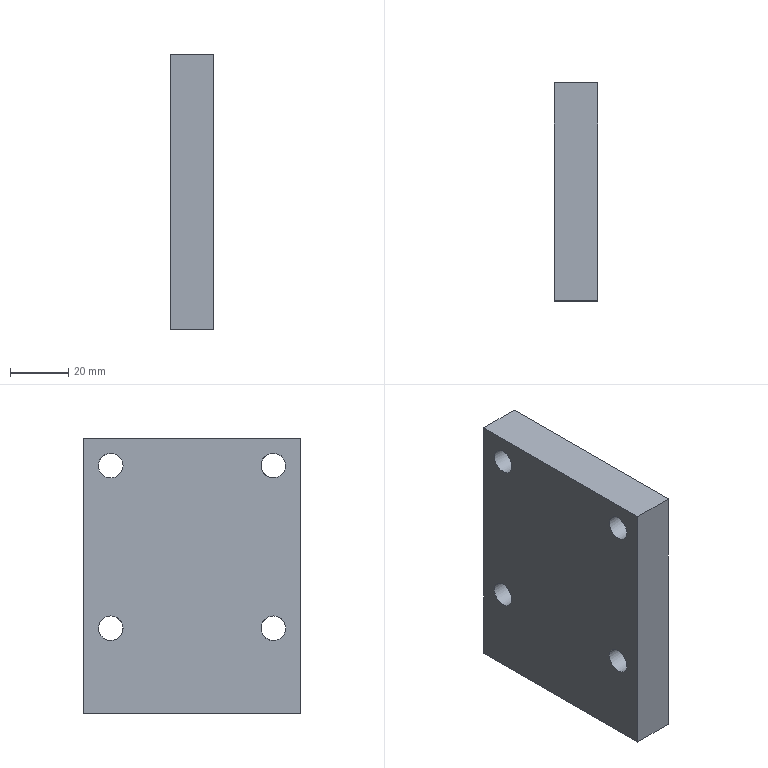Part | STEP file | Tube feed_id574_x_t | 1 solid | 18 faces | box 15 x 75 x 95 mm | volume 99971 mm3 | plane 10 | cylinder 8 | commonest cylinder face diameters 8.5 x4 14 x4
STEP:
#1=CARTESIAN_POINT('',(0.,0.,0.));
#2=DIRECTION('',(0.,0.,1.));
#3=DIRECTION('',(1.,0.,0.));
#4=AXIS2_PLACEMENT_3D('',#1,#2,#3);
#5=CARTESIAN_POINT('',(511.,506.436,-181.5));
#6=VERTEX_POINT('',#5);
#7=CARTESIAN_POINT('',(511.,506.436,-174.5));
#8=DIRECTION('',(-1.,0.,0.));
#9=DIRECTION('',(0.,0.,-1.));
#10=AXIS2_PLACEMENT_3D('',#7,#8,#9);
#11=CIRCLE('',#10,7.);
#12=CARTESIAN_POINT('',(511.,496.936,-204.));
#13=DIRECTION('',(1.,0.,0.));
#14=DIRECTION('',(0.,0.,-1.));
#15=AXIS2_PLACEMENT_3D('',#12,#13,#14);
#16=PLANE('',#15);
#17=CARTESIAN_POINT('',(-22.5,9.5));
#18=CARTESIAN_POINT('',(-22.5,-2.624));
#19=CARTESIAN_POINT('',(-33.,3.438));
#20=CARTESIAN_POINT('',(-43.5,9.5));
#21=CARTESIAN_POINT('',(-33.,15.562));
#22=CARTESIAN_POINT('',(-22.5,21.624));
#23=CARTESIAN_POINT('',(-22.5,9.5));
#24=(BOUNDED_CURVE()B_SPLINE_CURVE(2,(#17,#18,#19,#20,#21,#22,#23),.UNSPECIFIED.,.T.,.F.)B_SPLINE_CURVE_WITH_KNOTS((1,2,2,2,2,1),(-2.094,0.,2.094,4.189,6.283,8.378),.UNSPECIFIED.)CURVE()GEOMETRIC_REPRESENTATION_ITEM()RATIONAL_B_SPLINE_CURVE((1.,0.5,1.,0.5,1.,0.5,1.))REPRESENTATION_ITEM(''));
#25=(GEOMETRIC_REPRESENTATION_CONTEXT(2)PARAMETRIC_REPRESENTATION_CONTEXT()REPRESENTATION_CONTEXT('',''));
#26=DEFINITIONAL_REPRESENTATION('',(#24),#25);
#27=PCURVE('',#16,#26);
#28=CARTESIAN_POINT('',(502.,506.436,-174.5));
#29=DIRECTION('',(1.,0.,0.));
#30=DIRECTION('',(0.,0.,-1.));
#31=AXIS2_PLACEMENT_3D('',#28,#29,#30);
#32=CYLINDRICAL_SURFACE('',#31,7.);
#33=CARTESIAN_POINT('',(6.283,9.));
#34=DIRECTION('',(-1.,0.));
#35=VECTOR('',#34,1.);
#36=LINE('',#33,#35);
#37=(GEOMETRIC_REPRESENTATION_CONTEXT(2)PARAMETRIC_REPRESENTATION_CONTEXT()REPRESENTATION_CONTEXT('',''));
#38=DEFINITIONAL_REPRESENTATION('',(#36),#37);
#39=PCURVE('',#32,#38);
#40=SURFACE_CURVE('',#11,(#27,#39),.PCURVE_S1.);
#41=EDGE_CURVE('',#6,#6,#40,.T.);
#42=ORIENTED_EDGE('',*,*,#41,.T.);
#43=EDGE_LOOP('',(#42));
#44=FACE_BOUND('',#43,.T.);
#45=CARTESIAN_POINT('',(511.,496.936,-109.));
#46=VERTEX_POINT('',#45);
#47=CARTESIAN_POINT('',(511.,571.936,-109.));
#48=VERTEX_POINT('',#47);
#49=CARTESIAN_POINT('',(511.,496.936,-109.));
#50=DIRECTION('',(0.,1.,0.));
#51=VECTOR('',#50,1.);
#52=LINE('',#49,#51);
#53=CARTESIAN_POINT('',(-95.,0.));
#54=DIRECTION('',(0.,1.));
#55=VECTOR('',#54,1.);
#56=LINE('',#53,#55);
#57=(GEOMETRIC_REPRESENTATION_CONTEXT(2)PARAMETRIC_REPRESENTATION_CONTEXT()REPRESENTATION_CONTEXT('',''));
#58=DEFINITIONAL_REPRESENTATION('',(#56),#57);
#59=PCURVE('',#16,#58);
#60=CARTESIAN_POINT('',(0.,0.,-109.));
#61=DIRECTION('',(0.,0.,1.));
#62=DIRECTION('',(1.,0.,0.));
#63=AXIS2_PLACEMENT_3D('',#60,#61,#62);
#64=PLANE('',#63);
#65=CARTESIAN_POINT('',(511.,496.936));
#66=DIRECTION('',(0.,1.));
#67=VECTOR('',#66,1.);
#68=LINE('',#65,#67);
#69=(GEOMETRIC_REPRESENTATION_CONTEXT(2)PARAMETRIC_REPRESENTATION_CONTEXT()REPRESENTATION_CONTEXT('',''));
#70=DEFINITIONAL_REPRESENTATION('',(#68),#69);
#71=PCURVE('',#64,#70);
#72=SURFACE_CURVE('',#52,(#59,#71),.PCURVE_S1.);
#73=EDGE_CURVE('',#46,#48,#72,.T.);
#74=ORIENTED_EDGE('',*,*,#73,.F.);
#75=CARTESIAN_POINT('',(511.,496.936,-204.));
#76=VERTEX_POINT('',#75);
#77=CARTESIAN_POINT('',(511.,496.936,-204.));
#78=DIRECTION('',(0.,0.,1.));
#79=VECTOR('',#78,1.);
#80=LINE('',#77,#79);
#81=CARTESIAN_POINT('',(0.,0.));
#82=DIRECTION('',(-1.,0.));
#83=VECTOR('',#82,1.);
#84=LINE('',#81,#83);
#85=(GEOMETRIC_REPRESENTATION_CONTEXT(2)PARAMETRIC_REPRESENTATION_CONTEXT()REPRESENTATION_CONTEXT('',''));
#86=DEFINITIONAL_REPRESENTATION('',(#84),#85);
#87=PCURVE('',#16,#86);
#88=CARTESIAN_POINT('',(496.,496.936,-204.));
#89=DIRECTION('',(0.,-1.,0.));
#90=DIRECTION('',(1.,0.,0.));
#91=AXIS2_PLACEMENT_3D('',#88,#89,#90);
#92=PLANE('',#91);
#93=CARTESIAN_POINT('',(15.,0.));
#94=DIRECTION('',(0.,1.));
#95=VECTOR('',#94,1.);
#96=LINE('',#93,#95);
#97=(GEOMETRIC_REPRESENTATION_CONTEXT(2)PARAMETRIC_REPRESENTATION_CONTEXT()REPRESENTATION_CONTEXT('',''));
#98=DEFINITIONAL_REPRESENTATION('',(#96),#97);
#99=PCURVE('',#92,#98);
#100=SURFACE_CURVE('',#80,(#87,#99),.PCURVE_S1.);
#101=EDGE_CURVE('',#76,#46,#100,.T.);
#102=ORIENTED_EDGE('',*,*,#101,.F.);
#103=CARTESIAN_POINT('',(511.,571.936,-204.));
#104=VERTEX_POINT('',#103);
#105=CARTESIAN_POINT('',(511.,496.936,-204.));
#106=DIRECTION('',(0.,1.,0.));
#107=VECTOR('',#106,1.);
#108=LINE('',#105,#107);
#109=CARTESIAN_POINT('',(0.,0.));
#110=DIRECTION('',(0.,1.));
#111=VECTOR('',#110,1.);
#112=LINE('',#109,#111);
#113=(GEOMETRIC_REPRESENTATION_CONTEXT(2)PARAMETRIC_REPRESENTATION_CONTEXT()REPRESENTATION_CONTEXT('',''));
#114=DEFINITIONAL_REPRESENTATION('',(#112),#113);
#115=PCURVE('',#16,#114);
#116=CARTESIAN_POINT('',(0.,0.,-204.));
#117=DIRECTION('',(0.,0.,1.));
#118=DIRECTION('',(1.,0.,0.));
#119=AXIS2_PLACEMENT_3D('',#116,#117,#118);
#120=PLANE('',#119);
#121=CARTESIAN_POINT('',(511.,496.936));
#122=DIRECTION('',(0.,1.));
#123=VECTOR('',#122,1.);
#124=LINE('',#121,#123);
#125=(GEOMETRIC_REPRESENTATION_CONTEXT(2)PARAMETRIC_REPRESENTATION_CONTEXT()REPRESENTATION_CONTEXT('',''));
#126=DEFINITIONAL_REPRESENTATION('',(#124),#125);
#127=PCURVE('',#120,#126);
#128=SURFACE_CURVE('',#108,(#115,#127),.PCURVE_S1.);
#129=EDGE_CURVE('',#76,#104,#128,.T.);
#130=ORIENTED_EDGE('',*,*,#129,.T.);
#131=CARTESIAN_POINT('',(511.,571.936,-204.));
#132=DIRECTION('',(0.,0.,1.));
#133=VECTOR('',#132,1.);
#134=LINE('',#131,#133);
#135=CARTESIAN_POINT('',(0.,75.));
#136=DIRECTION('',(-1.,0.));
#137=VECTOR('',#136,1.);
#138=LINE('',#135,#137);
#139=(GEOMETRIC_REPRESENTATION_CONTEXT(2)PARAMETRIC_REPRESENTATION_CONTEXT()REPRESENTATION_CONTEXT('',''));
#140=DEFINITIONAL_REPRESENTATION('',(#138),#139);
#141=PCURVE('',#16,#140);
#142=CARTESIAN_POINT('',(511.,571.936,-204.));
#143=DIRECTION('',(0.,1.,0.));
#144=DIRECTION('',(0.,0.,1.));
#145=AXIS2_PLACEMENT_3D('',#142,#143,#144);
#146=PLANE('',#145);
#147=CARTESIAN_POINT('',(0.,0.));
#148=DIRECTION('',(1.,0.));
#149=VECTOR('',#148,1.);
#150=LINE('',#147,#149);
#151=(GEOMETRIC_REPRESENTATION_CONTEXT(2)PARAMETRIC_REPRESENTATION_CONTEXT()REPRESENTATION_CONTEXT('',''));
#152=DEFINITIONAL_REPRESENTATION('',(#150),#151);
#153=PCURVE('',#146,#152);
#154=SURFACE_CURVE('',#134,(#141,#153),.PCURVE_S1.);
#155=EDGE_CURVE('',#104,#48,#154,.T.);
#156=ORIENTED_EDGE('',*,*,#155,.T.);
#157=EDGE_LOOP('',(#74,#102,#130,#156));
#158=FACE_BOUND('',#157,.T.);
#159=CARTESIAN_POINT('',(511.,562.436,-125.5));
#160=VERTEX_POINT('',#159);
#161=CARTESIAN_POINT('',(511.,562.436,-118.5));
#162=DIRECTION('',(1.,0.,0.));
#163=DIRECTION('',(0.,0.,-1.));
#164=AXIS2_PLACEMENT_3D('',#161,#162,#163);
#165=CIRCLE('',#164,7.);
#166=CARTESIAN_POINT('',(-85.5,65.5));
#167=DIRECTION('',(1.,0.));
#168=AXIS2_PLACEMENT_2D('',#166,#167);
#169=CIRCLE('',#168,7.);
#170=(GEOMETRIC_REPRESENTATION_CONTEXT(2)PARAMETRIC_REPRESENTATION_CONTEXT()REPRESENTATION_CONTEXT('',''));
#171=DEFINITIONAL_REPRESENTATION('',(#169),#170);
#172=PCURVE('',#16,#171);
#173=CARTESIAN_POINT('',(502.,562.436,-118.5));
#174=DIRECTION('',(1.,0.,0.));
#175=DIRECTION('',(0.,0.,-1.));
#176=AXIS2_PLACEMENT_3D('',#173,#174,#175);
#177=CYLINDRICAL_SURFACE('',#176,7.);
#178=CARTESIAN_POINT('',(0.,9.));
#179=DIRECTION('',(1.,0.));
#180=VECTOR('',#179,1.);
#181=LINE('',#178,#180);
#182=(GEOMETRIC_REPRESENTATION_CONTEXT(2)PARAMETRIC_REPRESENTATION_CONTEXT()REPRESENTATION_CONTEXT('',''));
#183=DEFINITIONAL_REPRESENTATION('',(#181),#182);
#184=PCURVE('',#177,#183);
#185=SURFACE_CURVE('',#165,(#172,#184),.PCURVE_S1.);
#186=EDGE_CURVE('',#160,#160,#185,.T.);
#187=ORIENTED_EDGE('',*,*,#186,.F.);
#188=EDGE_LOOP('',(#187));
#189=FACE_BOUND('',#188,.T.);
#190=CARTESIAN_POINT('',(511.,506.436,-125.5));
#191=VERTEX_POINT('',#190);
#192=CARTESIAN_POINT('',(511.,506.436,-118.5));
#193=DIRECTION('',(-1.,0.,0.));
#194=DIRECTION('',(0.,0.,-1.));
#195=AXIS2_PLACEMENT_3D('',#192,#193,#194);
#196=CIRCLE('',#195,7.);
#197=CARTESIAN_POINT('',(-78.5,9.5));
#198=CARTESIAN_POINT('',(-78.5,-2.624));
#199=CARTESIAN_POINT('',(-89.,3.438));
#200=CARTESIAN_POINT('',(-99.5,9.5));
#201=CARTESIAN_POINT('',(-89.,15.562));
#202=CARTESIAN_POINT('',(-78.5,21.624));
#203=CARTESIAN_POINT('',(-78.5,9.5));
#204=(BOUNDED_CURVE()B_SPLINE_CURVE(2,(#197,#198,#199,#200,#201,#202,#203),.UNSPECIFIED.,.T.,.F.)B_SPLINE_CURVE_WITH_KNOTS((1,2,2,2,2,1),(-2.094,0.,2.094,4.189,6.283,8.378),.UNSPECIFIED.)CURVE()GEOMETRIC_REPRESENTATION_ITEM()RATIONAL_B_SPLINE_CURVE((1.,0.5,1.,0.5,1.,0.5,1.))REPRESENTATION_ITEM(''));
#205=(GEOMETRIC_REPRESENTATION_CONTEXT(2)PARAMETRIC_REPRESENTATION_CONTEXT()REPRESENTATION_CONTEXT('',''));
#206=DEFINITIONAL_REPRESENTATION('',(#204),#205);
#207=PCURVE('',#16,#206);
#208=CARTESIAN_POINT('',(502.,506.436,-118.5));
#209=DIRECTION('',(1.,0.,0.));
#210=DIRECTION('',(0.,0.,-1.));
#211=AXIS2_PLACEMENT_3D('',#208,#209,#210);
#212=CYLINDRICAL_SURFACE('',#211,7.);
#213=CARTESIAN_POINT('',(6.283,9.));
#214=DIRECTION('',(-1.,0.));
#215=VECTOR('',#214,1.);
#216=LINE('',#213,#215);
#217=(GEOMETRIC_REPRESENTATION_CONTEXT(2)PARAMETRIC_REPRESENTATION_CONTEXT()REPRESENTATION_CONTEXT('',''));
#218=DEFINITIONAL_REPRESENTATION('',(#216),#217);
#219=PCURVE('',#212,#218);
#220=SURFACE_CURVE('',#196,(#207,#219),.PCURVE_S1.);
#221=EDGE_CURVE('',#191,#191,#220,.T.);
#222=ORIENTED_EDGE('',*,*,#221,.T.);
#223=EDGE_LOOP('',(#222));
#224=FACE_BOUND('',#223,.T.);
#225=CARTESIAN_POINT('',(511.,562.436,-181.5));
#226=VERTEX_POINT('',#225);
#227=CARTESIAN_POINT('',(511.,562.436,-174.5));
#228=DIRECTION('',(-1.,0.,0.));
#229=DIRECTION('',(0.,0.,-1.));
#230=AXIS2_PLACEMENT_3D('',#227,#228,#229);
#231=CIRCLE('',#230,7.);
#232=CARTESIAN_POINT('',(-22.5,65.5));
#233=CARTESIAN_POINT('',(-22.5,53.376));
#234=CARTESIAN_POINT('',(-33.,59.438));
#235=CARTESIAN_POINT('',(-43.5,65.5));
#236=CARTESIAN_POINT('',(-33.,71.562));
#237=CARTESIAN_POINT('',(-22.5,77.624));
#238=CARTESIAN_POINT('',(-22.5,65.5));
#239=(BOUNDED_CURVE()B_SPLINE_CURVE(2,(#232,#233,#234,#235,#236,#237,#238),.UNSPECIFIED.,.T.,.F.)B_SPLINE_CURVE_WITH_KNOTS((1,2,2,2,2,1),(-2.094,0.,2.094,4.189,6.283,8.378),.UNSPECIFIED.)CURVE()GEOMETRIC_REPRESENTATION_ITEM()RATIONAL_B_SPLINE_CURVE((1.,0.5,1.,0.5,1.,0.5,1.))REPRESENTATION_ITEM(''));
#240=(GEOMETRIC_REPRESENTATION_CONTEXT(2)PARAMETRIC_REPRESENTATION_CONTEXT()REPRESENTATION_CONTEXT('',''));
#241=DEFINITIONAL_REPRESENTATION('',(#239),#240);
#242=PCURVE('',#16,#241);
#243=CARTESIAN_POINT('',(502.,562.436,-174.5));
#244=DIRECTION('',(1.,0.,0.));
#245=DIRECTION('',(0.,0.,-1.));
#246=AXIS2_PLACEMENT_3D('',#243,#244,#245);
#247=CYLINDRICAL_SURFACE('',#246,7.);
#248=CARTESIAN_POINT('',(6.283,9.));
#249=DIRECTION('',(-1.,0.));
#250=VECTOR('',#249,1.);
#251=LINE('',#248,#250);
#252=(GEOMETRIC_REPRESENTATION_CONTEXT(2)PARAMETRIC_REPRESENTATION_CONTEXT()REPRESENTATION_CONTEXT('',''));
#253=DEFINITIONAL_REPRESENTATION('',(#251),#252);
#254=PCURVE('',#247,#253);
#255=SURFACE_CURVE('',#231,(#242,#254),.PCURVE_S1.);
#256=EDGE_CURVE('',#226,#226,#255,.T.);
#257=ORIENTED_EDGE('',*,*,#256,.T.);
#258=EDGE_LOOP('',(#257));
#259=FACE_BOUND('',#258,.T.);
#260=ADVANCED_FACE('',(#44,#158,#189,#224,#259),#16,.T.);
#261=CARTESIAN_POINT('',(496.,558.186,-118.5));
#262=VERTEX_POINT('',#261);
#263=CARTESIAN_POINT('',(496.,562.436,-118.5));
#264=DIRECTION('',(1.,0.,0.));
#265=DIRECTION('',(0.,-1.,0.));
#266=AXIS2_PLACEMENT_3D('',#263,#264,#265);
#267=CIRCLE('',#266,4.25);
#268=CARTESIAN_POINT('',(569.4,562.436,-118.5));
#269=DIRECTION('',(-1.,0.,0.));
#270=DIRECTION('',(0.,0.,1.));
#271=AXIS2_PLACEMENT_3D('',#268,#269,#270);
#272=CYLINDRICAL_SURFACE('',#271,4.25);
#273=CARTESIAN_POINT('',(10.996,73.4));
#274=DIRECTION('',(-1.,0.));
#275=VECTOR('',#274,1.);
#276=LINE('',#273,#275);
#277=(GEOMETRIC_REPRESENTATION_CONTEXT(2)PARAMETRIC_REPRESENTATION_CONTEXT()REPRESENTATION_CONTEXT('',''));
#278=DEFINITIONAL_REPRESENTATION('',(#276),#277);
#279=PCURVE('',#272,#278);
#280=CARTESIAN_POINT('',(496.,571.936,-204.));
#281=DIRECTION('',(-1.,0.,0.));
#282=DIRECTION('',(0.,-1.,0.));
#283=AXIS2_PLACEMENT_3D('',#280,#281,#282);
#284=PLANE('',#283);
#285=CARTESIAN_POINT('',(13.75,85.5));
#286=CARTESIAN_POINT('',(13.75,78.139));
#287=CARTESIAN_POINT('',(7.375,81.819));
#288=CARTESIAN_POINT('',(1.,85.5));
#289=CARTESIAN_POINT('',(7.375,89.181));
#290=CARTESIAN_POINT('',(13.75,92.861));
#291=CARTESIAN_POINT('',(13.75,85.5));
#292=(BOUNDED_CURVE()B_SPLINE_CURVE(2,(#285,#286,#287,#288,#289,#290,#291),.UNSPECIFIED.,.T.,.F.)B_SPLINE_CURVE_WITH_KNOTS((1,2,2,2,2,1),(-2.094,0.,2.094,4.189,6.283,8.378),.UNSPECIFIED.)CURVE()GEOMETRIC_REPRESENTATION_ITEM()RATIONAL_B_SPLINE_CURVE((1.,0.5,1.,0.5,1.,0.5,1.))REPRESENTATION_ITEM(''));
#293=(GEOMETRIC_REPRESENTATION_CONTEXT(2)PARAMETRIC_REPRESENTATION_CONTEXT()REPRESENTATION_CONTEXT('',''));
#294=DEFINITIONAL_REPRESENTATION('',(#292),#293);
#295=PCURVE('',#284,#294);
#296=SURFACE_CURVE('',#267,(#279,#295),.PCURVE_S1.);
#297=EDGE_CURVE('',#262,#262,#296,.T.);
#298=ORIENTED_EDGE('',*,*,#297,.T.);
#299=CARTESIAN_POINT('',(502.,558.186,-118.5));
#300=VERTEX_POINT('',#299);
#301=CARTESIAN_POINT('',(502.,558.186,-118.5));
#302=CARTESIAN_POINT('',(496.,558.186,-118.5));
#303=B_SPLINE_CURVE_WITH_KNOTS('',1,(#301,#302),.UNSPECIFIED.,.F.,.F.,(2,2),(67.4,73.4),.PIECEWISE_BEZIER_KNOTS.);
#304=CARTESIAN_POINT('',(4.712,0.));
#305=DIRECTION('',(0.,1.));
#306=VECTOR('',#305,1.);
#307=LINE('',#304,#306);
#308=(GEOMETRIC_REPRESENTATION_CONTEXT(2)PARAMETRIC_REPRESENTATION_CONTEXT()REPRESENTATION_CONTEXT('',''));
#309=DEFINITIONAL_REPRESENTATION('',(#307),#308);
#310=PCURVE('',#272,#309);
#311=CARTESIAN_POINT('',(10.996,0.));
#312=DIRECTION('',(0.,1.));
#313=VECTOR('',#312,1.);
#314=LINE('',#311,#313);
#315=(GEOMETRIC_REPRESENTATION_CONTEXT(2)PARAMETRIC_REPRESENTATION_CONTEXT()REPRESENTATION_CONTEXT('',''));
#316=DEFINITIONAL_REPRESENTATION('',(#314),#315);
#317=PCURVE('',#272,#316);
#318=SEAM_CURVE('',#303,(#310,#317),.PCURVE_S1.);
#319=EDGE_CURVE('',#300,#262,#318,.T.);
#320=ORIENTED_EDGE('',*,*,#319,.F.);
#321=CARTESIAN_POINT('',(502.,562.436,-122.75));
#322=VERTEX_POINT('',#321);
#323=CARTESIAN_POINT('',(502.,562.436,-118.5));
#324=DIRECTION('',(1.,0.,0.));
#325=DIRECTION('',(0.,0.,-1.));
#326=AXIS2_PLACEMENT_3D('',#323,#324,#325);
#327=CIRCLE('',#326,4.25);
#328=CARTESIAN_POINT('',(9.425,67.4));
#329=DIRECTION('',(-1.,0.));
#330=VECTOR('',#329,1.);
#331=LINE('',#328,#330);
#332=(GEOMETRIC_REPRESENTATION_CONTEXT(2)PARAMETRIC_REPRESENTATION_CONTEXT()REPRESENTATION_CONTEXT('',''));
#333=DEFINITIONAL_REPRESENTATION('',(#331),#332);
#334=PCURVE('',#272,#333);
#335=CARTESIAN_POINT('',(502.,562.436,-118.5));
#336=DIRECTION('',(1.,0.,0.));
#337=DIRECTION('',(0.,0.,-1.));
#338=AXIS2_PLACEMENT_3D('',#335,#336,#337);
#339=PLANE('',#338);
#340=CARTESIAN_POINT('',(0.,0.));
#341=DIRECTION('',(1.,0.));
#342=AXIS2_PLACEMENT_2D('',#340,#341);
#343=CIRCLE('',#342,4.25);
#344=(GEOMETRIC_REPRESENTATION_CONTEXT(2)PARAMETRIC_REPRESENTATION_CONTEXT()REPRESENTATION_CONTEXT('',''));
#345=DEFINITIONAL_REPRESENTATION('',(#343),#344);
#346=PCURVE('',#339,#345);
#347=SURFACE_CURVE('',#327,(#334,#346),.PCURVE_S1.);
#348=EDGE_CURVE('',#322,#300,#347,.T.);
#349=ORIENTED_EDGE('',*,*,#348,.F.);
#350=CARTESIAN_POINT('',(502.,562.436,-118.5));
#351=DIRECTION('',(1.,0.,0.));
#352=DIRECTION('',(0.,0.,-1.));
#353=AXIS2_PLACEMENT_3D('',#350,#351,#352);
#354=CIRCLE('',#353,4.25);
#355=CARTESIAN_POINT('',(15.708,67.4));
#356=DIRECTION('',(-1.,0.));
#357=VECTOR('',#356,1.);
#358=LINE('',#355,#357);
#359=(GEOMETRIC_REPRESENTATION_CONTEXT(2)PARAMETRIC_REPRESENTATION_CONTEXT()REPRESENTATION_CONTEXT('',''));
#360=DEFINITIONAL_REPRESENTATION('',(#358),#359);
#361=PCURVE('',#272,#360);
#362=CARTESIAN_POINT('',(0.,0.));
#363=DIRECTION('',(1.,0.));
#364=AXIS2_PLACEMENT_2D('',#362,#363);
#365=CIRCLE('',#364,4.25);
#366=(GEOMETRIC_REPRESENTATION_CONTEXT(2)PARAMETRIC_REPRESENTATION_CONTEXT()REPRESENTATION_CONTEXT('',''));
#367=DEFINITIONAL_REPRESENTATION('',(#365),#366);
#368=PCURVE('',#339,#367);
#369=SURFACE_CURVE('',#354,(#361,#368),.PCURVE_S1.);
#370=EDGE_CURVE('',#300,#322,#369,.T.);
#371=ORIENTED_EDGE('',*,*,#370,.F.);
#372=ORIENTED_EDGE('',*,*,#319,.T.);
#373=EDGE_LOOP('',(#298,#320,#349,#371,#372));
#374=FACE_BOUND('',#373,.F.);
#375=ADVANCED_FACE('',(#374),#272,.F.);
#376=CARTESIAN_POINT('',(496.,558.186,-174.5));
#377=VERTEX_POINT('',#376);
#378=CARTESIAN_POINT('',(496.,562.436,-170.25));
#379=VERTEX_POINT('',#378);
#380=CARTESIAN_POINT('',(496.,562.436,-174.5));
#381=DIRECTION('',(1.,0.,0.));
#382=DIRECTION('',(0.,-1.,0.));
#383=AXIS2_PLACEMENT_3D('',#380,#381,#382);
#384=CIRCLE('',#383,4.25);
#385=CARTESIAN_POINT('',(13.75,29.5));
#386=CARTESIAN_POINT('',(13.75,22.139));
#387=CARTESIAN_POINT('',(7.375,25.819));
#388=CARTESIAN_POINT('',(1.,29.5));
#389=CARTESIAN_POINT('',(7.375,33.181));
#390=CARTESIAN_POINT('',(13.75,36.861));
#391=CARTESIAN_POINT('',(13.75,29.5));
#392=(BOUNDED_CURVE()B_SPLINE_CURVE(2,(#385,#386,#387,#388,#389,#390,#391),.UNSPECIFIED.,.T.,.F.)B_SPLINE_CURVE_WITH_KNOTS((1,2,2,2,2,1),(-2.094,0.,2.094,4.189,6.283,8.378),.UNSPECIFIED.)CURVE()GEOMETRIC_REPRESENTATION_ITEM()RATIONAL_B_SPLINE_CURVE((1.,0.5,1.,0.5,1.,0.5,1.))REPRESENTATION_ITEM(''));
#393=(GEOMETRIC_REPRESENTATION_CONTEXT(2)PARAMETRIC_REPRESENTATION_CONTEXT()REPRESENTATION_CONTEXT('',''));
#394=DEFINITIONAL_REPRESENTATION('',(#392),#393);
#395=PCURVE('',#284,#394);
#396=CARTESIAN_POINT('',(569.4,562.436,-174.5));
#397=DIRECTION('',(-1.,0.,0.));
#398=DIRECTION('',(0.,0.,1.));
#399=AXIS2_PLACEMENT_3D('',#396,#397,#398);
#400=CYLINDRICAL_SURFACE('',#399,4.25);
#401=CARTESIAN_POINT('',(4.712,73.4));
#402=DIRECTION('',(-1.,0.));
#403=VECTOR('',#402,1.);
#404=LINE('',#401,#403);
#405=(GEOMETRIC_REPRESENTATION_CONTEXT(2)PARAMETRIC_REPRESENTATION_CONTEXT()REPRESENTATION_CONTEXT('',''));
#406=DEFINITIONAL_REPRESENTATION('',(#404),#405);
#407=PCURVE('',#400,#406);
#408=SURFACE_CURVE('',#384,(#395,#407),.PCURVE_S1.);
#409=EDGE_CURVE('',#377,#379,#408,.T.);
#410=ORIENTED_EDGE('',*,*,#409,.T.);
#411=CARTESIAN_POINT('',(496.,562.436,-174.5));
#412=DIRECTION('',(1.,0.,0.));
#413=DIRECTION('',(0.,-1.,0.));
#414=AXIS2_PLACEMENT_3D('',#411,#412,#413);
#415=CIRCLE('',#414,4.25);
#416=CARTESIAN_POINT('',(13.75,29.5));
#417=CARTESIAN_POINT('',(13.75,22.139));
#418=CARTESIAN_POINT('',(7.375,25.819));
#419=CARTESIAN_POINT('',(1.,29.5));
#420=CARTESIAN_POINT('',(7.375,33.181));
#421=CARTESIAN_POINT('',(13.75,36.861));
#422=CARTESIAN_POINT('',(13.75,29.5));
#423=(BOUNDED_CURVE()B_SPLINE_CURVE(2,(#416,#417,#418,#419,#420,#421,#422),.UNSPECIFIED.,.T.,.F.)B_SPLINE_CURVE_WITH_KNOTS((1,2,2,2,2,1),(-2.094,0.,2.094,4.189,6.283,8.378),.UNSPECIFIED.)CURVE()GEOMETRIC_REPRESENTATION_ITEM()RATIONAL_B_SPLINE_CURVE((1.,0.5,1.,0.5,1.,0.5,1.))REPRESENTATION_ITEM(''));
#424=(GEOMETRIC_REPRESENTATION_CONTEXT(2)PARAMETRIC_REPRESENTATION_CONTEXT()REPRESENTATION_CONTEXT('',''));
#425=DEFINITIONAL_REPRESENTATION('',(#423),#424);
#426=PCURVE('',#284,#425);
#427=CARTESIAN_POINT('',(10.996,73.4));
#428=DIRECTION('',(-1.,0.));
#429=VECTOR('',#428,1.);
#430=LINE('',#427,#429);
#431=(GEOMETRIC_REPRESENTATION_CONTEXT(2)PARAMETRIC_REPRESENTATION_CONTEXT()REPRESENTATION_CONTEXT('',''));
#432=DEFINITIONAL_REPRESENTATION('',(#430),#431);
#433=PCURVE('',#400,#432);
#434=SURFACE_CURVE('',#415,(#426,#433),.PCURVE_S1.);
#435=EDGE_CURVE('',#379,#377,#434,.T.);
#436=ORIENTED_EDGE('',*,*,#435,.T.);
#437=EDGE_LOOP('',(#410,#436));
#438=FACE_BOUND('',#437,.T.);
#439=CARTESIAN_POINT('',(496.,502.186,-118.5));
#440=VERTEX_POINT('',#439);
#441=CARTESIAN_POINT('',(496.,506.436,-114.25));
#442=VERTEX_POINT('',#441);
#443=CARTESIAN_POINT('',(496.,506.436,-118.5));
#444=DIRECTION('',(1.,0.,0.));
#445=DIRECTION('',(0.,-1.,0.));
#446=AXIS2_PLACEMENT_3D('',#443,#444,#445);
#447=CIRCLE('',#446,4.25);
#448=CARTESIAN_POINT('',(69.75,85.5));
#449=CARTESIAN_POINT('',(69.75,78.139));
#450=CARTESIAN_POINT('',(63.375,81.819));
#451=CARTESIAN_POINT('',(57.,85.5));
#452=CARTESIAN_POINT('',(63.375,89.181));
#453=CARTESIAN_POINT('',(69.75,92.861));
#454=CARTESIAN_POINT('',(69.75,85.5));
#455=(BOUNDED_CURVE()B_SPLINE_CURVE(2,(#448,#449,#450,#451,#452,#453,#454),.UNSPECIFIED.,.T.,.F.)B_SPLINE_CURVE_WITH_KNOTS((1,2,2,2,2,1),(-2.094,0.,2.094,4.189,6.283,8.378),.UNSPECIFIED.)CURVE()GEOMETRIC_REPRESENTATION_ITEM()RATIONAL_B_SPLINE_CURVE((1.,0.5,1.,0.5,1.,0.5,1.))REPRESENTATION_ITEM(''));
#456=(GEOMETRIC_REPRESENTATION_CONTEXT(2)PARAMETRIC_REPRESENTATION_CONTEXT()REPRESENTATION_CONTEXT('',''));
#457=DEFINITIONAL_REPRESENTATION('',(#455),#456);
#458=PCURVE('',#284,#457);
#459=CARTESIAN_POINT('',(569.4,506.436,-118.5));
#460=DIRECTION('',(-1.,0.,0.));
#461=DIRECTION('',(0.,0.,1.));
#462=AXIS2_PLACEMENT_3D('',#459,#460,#461);
#463=CYLINDRICAL_SURFACE('',#462,4.25);
#464=CARTESIAN_POINT('',(4.712,73.4));
#465=DIRECTION('',(-1.,0.));
#466=VECTOR('',#465,1.);
#467=LINE('',#464,#466);
#468=(GEOMETRIC_REPRESENTATION_CONTEXT(2)PARAMETRIC_REPRESENTATION_CONTEXT()REPRESENTATION_CONTEXT('',''));
#469=DEFINITIONAL_REPRESENTATION('',(#467),#468);
#470=PCURVE('',#463,#469);
#471=SURFACE_CURVE('',#447,(#458,#470),.PCURVE_S1.);
#472=EDGE_CURVE('',#440,#442,#471,.T.);
#473=ORIENTED_EDGE('',*,*,#472,.T.);
#474=CARTESIAN_POINT('',(496.,506.436,-118.5));
#475=DIRECTION('',(1.,0.,0.));
#476=DIRECTION('',(0.,-1.,0.));
#477=AXIS2_PLACEMENT_3D('',#474,#475,#476);
#478=CIRCLE('',#477,4.25);
#479=CARTESIAN_POINT('',(69.75,85.5));
#480=CARTESIAN_POINT('',(69.75,78.139));
#481=CARTESIAN_POINT('',(63.375,81.819));
#482=CARTESIAN_POINT('',(57.,85.5));
#483=CARTESIAN_POINT('',(63.375,89.181));
#484=CARTESIAN_POINT('',(69.75,92.861));
#485=CARTESIAN_POINT('',(69.75,85.5));
#486=(BOUNDED_CURVE()B_SPLINE_CURVE(2,(#479,#480,#481,#482,#483,#484,#485),.UNSPECIFIED.,.T.,.F.)B_SPLINE_CURVE_WITH_KNOTS((1,2,2,2,2,1),(-2.094,0.,2.094,4.189,6.283,8.378),.UNSPECIFIED.)CURVE()GEOMETRIC_REPRESENTATION_ITEM()RATIONAL_B_SPLINE_CURVE((1.,0.5,1.,0.5,1.,0.5,1.))REPRESENTATION_ITEM(''));
#487=(GEOMETRIC_REPRESENTATION_CONTEXT(2)PARAMETRIC_REPRESENTATION_CONTEXT()REPRESENTATION_CONTEXT('',''));
#488=DEFINITIONAL_REPRESENTATION('',(#486),#487);
#489=PCURVE('',#284,#488);
#490=CARTESIAN_POINT('',(10.996,73.4));
#491=DIRECTION('',(-1.,0.));
#492=VECTOR('',#491,1.);
#493=LINE('',#490,#492);
#494=(GEOMETRIC_REPRESENTATION_CONTEXT(2)PARAMETRIC_REPRESENTATION_CONTEXT()REPRESENTATION_CONTEXT('',''));
#495=DEFINITIONAL_REPRESENTATION('',(#493),#494);
#496=PCURVE('',#463,#495);
#497=SURFACE_CURVE('',#478,(#489,#496),.PCURVE_S1.);
#498=EDGE_CURVE('',#442,#440,#497,.T.);
#499=ORIENTED_EDGE('',*,*,#498,.T.);
#500=EDGE_LOOP('',(#473,#499));
#501=FACE_BOUND('',#500,.T.);
#502=CARTESIAN_POINT('',(496.,502.186,-174.5));
#503=VERTEX_POINT('',#502);
#504=CARTESIAN_POINT('',(496.,506.436,-170.25));
#505=VERTEX_POINT('',#504);
#506=CARTESIAN_POINT('',(496.,506.436,-174.5));
#507=DIRECTION('',(1.,0.,0.));
#508=DIRECTION('',(0.,-1.,0.));
#509=AXIS2_PLACEMENT_3D('',#506,#507,#508);
#510=CIRCLE('',#509,4.25);
#511=CARTESIAN_POINT('',(69.75,29.5));
#512=CARTESIAN_POINT('',(69.75,22.139));
#513=CARTESIAN_POINT('',(63.375,25.819));
#514=CARTESIAN_POINT('',(57.,29.5));
#515=CARTESIAN_POINT('',(63.375,33.181));
#516=CARTESIAN_POINT('',(69.75,36.861));
#517=CARTESIAN_POINT('',(69.75,29.5));
#518=(BOUNDED_CURVE()B_SPLINE_CURVE(2,(#511,#512,#513,#514,#515,#516,#517),.UNSPECIFIED.,.T.,.F.)B_SPLINE_CURVE_WITH_KNOTS((1,2,2,2,2,1),(-2.094,0.,2.094,4.189,6.283,8.378),.UNSPECIFIED.)CURVE()GEOMETRIC_REPRESENTATION_ITEM()RATIONAL_B_SPLINE_CURVE((1.,0.5,1.,0.5,1.,0.5,1.))REPRESENTATION_ITEM(''));
#519=(GEOMETRIC_REPRESENTATION_CONTEXT(2)PARAMETRIC_REPRESENTATION_CONTEXT()REPRESENTATION_CONTEXT('',''));
#520=DEFINITIONAL_REPRESENTATION('',(#518),#519);
#521=PCURVE('',#284,#520);
#522=CARTESIAN_POINT('',(569.4,506.436,-174.5));
#523=DIRECTION('',(-1.,0.,0.));
#524=DIRECTION('',(0.,0.,1.));
#525=AXIS2_PLACEMENT_3D('',#522,#523,#524);
#526=CYLINDRICAL_SURFACE('',#525,4.25);
#527=CARTESIAN_POINT('',(4.712,73.4));
#528=DIRECTION('',(-1.,0.));
#529=VECTOR('',#528,1.);
#530=LINE('',#527,#529);
#531=(GEOMETRIC_REPRESENTATION_CONTEXT(2)PARAMETRIC_REPRESENTATION_CONTEXT()REPRESENTATION_CONTEXT('',''));
#532=DEFINITIONAL_REPRESENTATION('',(#530),#531);
#533=PCURVE('',#526,#532);
#534=SURFACE_CURVE('',#510,(#521,#533),.PCURVE_S1.);
#535=EDGE_CURVE('',#503,#505,#534,.T.);
#536=ORIENTED_EDGE('',*,*,#535,.T.);
#537=CARTESIAN_POINT('',(496.,506.436,-174.5));
#538=DIRECTION('',(1.,0.,0.));
#539=DIRECTION('',(0.,-1.,0.));
#540=AXIS2_PLACEMENT_3D('',#537,#538,#539);
#541=CIRCLE('',#540,4.25);
#542=CARTESIAN_POINT('',(69.75,29.5));
#543=CARTESIAN_POINT('',(69.75,22.139));
#544=CARTESIAN_POINT('',(63.375,25.819));
#545=CARTESIAN_POINT('',(57.,29.5));
#546=CARTESIAN_POINT('',(63.375,33.181));
#547=CARTESIAN_POINT('',(69.75,36.861));
#548=CARTESIAN_POINT('',(69.75,29.5));
#549=(BOUNDED_CURVE()B_SPLINE_CURVE(2,(#542,#543,#544,#545,#546,#547,#548),.UNSPECIFIED.,.T.,.F.)B_SPLINE_CURVE_WITH_KNOTS((1,2,2,2,2,1),(-2.094,0.,2.094,4.189,6.283,8.378),.UNSPECIFIED.)CURVE()GEOMETRIC_REPRESENTATION_ITEM()RATIONAL_B_SPLINE_CURVE((1.,0.5,1.,0.5,1.,0.5,1.))REPRESENTATION_ITEM(''));
#550=(GEOMETRIC_REPRESENTATION_CONTEXT(2)PARAMETRIC_REPRESENTATION_CONTEXT()REPRESENTATION_CONTEXT('',''));
#551=DEFINITIONAL_REPRESENTATION('',(#549),#550);
#552=PCURVE('',#284,#551);
#553=CARTESIAN_POINT('',(10.996,73.4));
#554=DIRECTION('',(-1.,0.));
#555=VECTOR('',#554,1.);
#556=LINE('',#553,#555);
#557=(GEOMETRIC_REPRESENTATION_CONTEXT(2)PARAMETRIC_REPRESENTATION_CONTEXT()REPRESENTATION_CONTEXT('',''));
#558=DEFINITIONAL_REPRESENTATION('',(#556),#557);
#559=PCURVE('',#526,#558);
#560=SURFACE_CURVE('',#541,(#552,#559),.PCURVE_S1.);
#561=EDGE_CURVE('',#505,#503,#560,.T.);
#562=ORIENTED_EDGE('',*,*,#561,.T.);
#563=EDGE_LOOP('',(#536,#562));
#564=FACE_BOUND('',#563,.T.);
#565=ORIENTED_EDGE('',*,*,#297,.T.);
#566=EDGE_LOOP('',(#565));
#567=FACE_BOUND('',#566,.T.);
#568=CARTESIAN_POINT('',(496.,571.936,-109.));
#569=VERTEX_POINT('',#568);
#570=CARTESIAN_POINT('',(496.,496.936,-109.));
#571=VERTEX_POINT('',#570);
#572=CARTESIAN_POINT('',(496.,571.936,-109.));
#573=DIRECTION('',(0.,-1.,0.));
#574=VECTOR('',#573,1.);
#575=LINE('',#572,#574);
#576=CARTESIAN_POINT('',(0.,95.));
#577=DIRECTION('',(1.,0.));
#578=VECTOR('',#577,1.);
#579=LINE('',#576,#578);
#580=(GEOMETRIC_REPRESENTATION_CONTEXT(2)PARAMETRIC_REPRESENTATION_CONTEXT()REPRESENTATION_CONTEXT('',''));
#581=DEFINITIONAL_REPRESENTATION('',(#579),#580);
#582=PCURVE('',#284,#581);
#583=CARTESIAN_POINT('',(496.,571.936));
#584=DIRECTION('',(0.,-1.));
#585=VECTOR('',#584,1.);
#586=LINE('',#583,#585);
#587=(GEOMETRIC_REPRESENTATION_CONTEXT(2)PARAMETRIC_REPRESENTATION_CONTEXT()REPRESENTATION_CONTEXT('',''));
#588=DEFINITIONAL_REPRESENTATION('',(#586),#587);
#589=PCURVE('',#64,#588);
#590=SURFACE_CURVE('',#575,(#582,#589),.PCURVE_S1.);
#591=EDGE_CURVE('',#569,#571,#590,.T.);
#592=ORIENTED_EDGE('',*,*,#591,.F.);
#593=CARTESIAN_POINT('',(496.,571.936,-204.));
#594=VERTEX_POINT('',#593);
#595=CARTESIAN_POINT('',(496.,571.936,-204.));
#596=DIRECTION('',(0.,0.,1.));
#597=VECTOR('',#596,1.);
#598=LINE('',#595,#597);
#599=CARTESIAN_POINT('',(0.,0.));
#600=DIRECTION('',(0.,1.));
#601=VECTOR('',#600,1.);
#602=LINE('',#599,#601);
#603=(GEOMETRIC_REPRESENTATION_CONTEXT(2)PARAMETRIC_REPRESENTATION_CONTEXT()REPRESENTATION_CONTEXT('',''));
#604=DEFINITIONAL_REPRESENTATION('',(#602),#603);
#605=PCURVE('',#284,#604);
#606=CARTESIAN_POINT('',(0.,-15.));
#607=DIRECTION('',(1.,0.));
#608=VECTOR('',#607,1.);
#609=LINE('',#606,#608);
#610=(GEOMETRIC_REPRESENTATION_CONTEXT(2)PARAMETRIC_REPRESENTATION_CONTEXT()REPRESENTATION_CONTEXT('',''));
#611=DEFINITIONAL_REPRESENTATION('',(#609),#610);
#612=PCURVE('',#146,#611);
#613=SURFACE_CURVE('',#598,(#605,#612),.PCURVE_S1.);
#614=EDGE_CURVE('',#594,#569,#613,.T.);
#615=ORIENTED_EDGE('',*,*,#614,.F.);
#616=CARTESIAN_POINT('',(496.,496.936,-204.));
#617=VERTEX_POINT('',#616);
#618=CARTESIAN_POINT('',(496.,571.936,-204.));
#619=DIRECTION('',(0.,-1.,0.));
#620=VECTOR('',#619,1.);
#621=LINE('',#618,#620);
#622=CARTESIAN_POINT('',(0.,0.));
#623=DIRECTION('',(1.,0.));
#624=VECTOR('',#623,1.);
#625=LINE('',#622,#624);
#626=(GEOMETRIC_REPRESENTATION_CONTEXT(2)PARAMETRIC_REPRESENTATION_CONTEXT()REPRESENTATION_CONTEXT('',''));
#627=DEFINITIONAL_REPRESENTATION('',(#625),#626);
#628=PCURVE('',#284,#627);
#629=CARTESIAN_POINT('',(496.,571.936));
#630=DIRECTION('',(0.,-1.));
#631=VECTOR('',#630,1.);
#632=LINE('',#629,#631);
#633=(GEOMETRIC_REPRESENTATION_CONTEXT(2)PARAMETRIC_REPRESENTATION_CONTEXT()REPRESENTATION_CONTEXT('',''));
#634=DEFINITIONAL_REPRESENTATION('',(#632),#633);
#635=PCURVE('',#120,#634);
#636=SURFACE_CURVE('',#621,(#628,#635),.PCURVE_S1.);
#637=EDGE_CURVE('',#594,#617,#636,.T.);
#638=ORIENTED_EDGE('',*,*,#637,.T.);
#639=CARTESIAN_POINT('',(496.,496.936,-204.));
#640=DIRECTION('',(0.,0.,1.));
#641=VECTOR('',#640,1.);
#642=LINE('',#639,#641);
#643=CARTESIAN_POINT('',(75.,0.));
#644=DIRECTION('',(0.,1.));
#645=VECTOR('',#644,1.);
#646=LINE('',#643,#645);
#647=(GEOMETRIC_REPRESENTATION_CONTEXT(2)PARAMETRIC_REPRESENTATION_CONTEXT()REPRESENTATION_CONTEXT('',''));
#648=DEFINITIONAL_REPRESENTATION('',(#646),#647);
#649=PCURVE('',#284,#648);
#650=CARTESIAN_POINT('',(0.,0.));
#651=DIRECTION('',(0.,1.));
#652=VECTOR('',#651,1.);
#653=LINE('',#650,#652);
#654=(GEOMETRIC_REPRESENTATION_CONTEXT(2)PARAMETRIC_REPRESENTATION_CONTEXT()REPRESENTATION_CONTEXT('',''));
#655=DEFINITIONAL_REPRESENTATION('',(#653),#654);
#656=PCURVE('',#92,#655);
#657=SURFACE_CURVE('',#642,(#649,#656),.PCURVE_S1.);
#658=EDGE_CURVE('',#617,#571,#657,.T.);
#659=ORIENTED_EDGE('',*,*,#658,.T.);
#660=EDGE_LOOP('',(#592,#615,#638,#659));
#661=FACE_BOUND('',#660,.T.);
#662=ADVANCED_FACE('',(#438,#501,#564,#567,#661),#284,.T.);
#663=CARTESIAN_POINT('',(496.,496.936,-109.));
#664=DIRECTION('',(1.,0.,0.));
#665=VECTOR('',#664,1.);
#666=LINE('',#663,#665);
#667=CARTESIAN_POINT('',(0.,95.));
#668=DIRECTION('',(1.,0.));
#669=VECTOR('',#668,1.);
#670=LINE('',#667,#669);
#671=(GEOMETRIC_REPRESENTATION_CONTEXT(2)PARAMETRIC_REPRESENTATION_CONTEXT()REPRESENTATION_CONTEXT('',''));
#672=DEFINITIONAL_REPRESENTATION('',(#670),#671);
#673=PCURVE('',#92,#672);
#674=CARTESIAN_POINT('',(496.,496.936));
#675=DIRECTION('',(1.,0.));
#676=VECTOR('',#675,1.);
#677=LINE('',#674,#676);
#678=(GEOMETRIC_REPRESENTATION_CONTEXT(2)PARAMETRIC_REPRESENTATION_CONTEXT()REPRESENTATION_CONTEXT('',''));
#679=DEFINITIONAL_REPRESENTATION('',(#677),#678);
#680=PCURVE('',#64,#679);
#681=SURFACE_CURVE('',#666,(#673,#680),.PCURVE_S1.);
#682=EDGE_CURVE('',#571,#46,#681,.T.);
#683=ORIENTED_EDGE('',*,*,#682,.F.);
#684=ORIENTED_EDGE('',*,*,#658,.F.);
#685=CARTESIAN_POINT('',(496.,496.936,-204.));
#686=DIRECTION('',(1.,0.,0.));
#687=VECTOR('',#686,1.);
#688=LINE('',#685,#687);
#689=CARTESIAN_POINT('',(0.,0.));
#690=DIRECTION('',(1.,0.));
#691=VECTOR('',#690,1.);
#692=LINE('',#689,#691);
#693=(GEOMETRIC_REPRESENTATION_CONTEXT(2)PARAMETRIC_REPRESENTATION_CONTEXT()REPRESENTATION_CONTEXT('',''));
#694=DEFINITIONAL_REPRESENTATION('',(#692),#693);
#695=PCURVE('',#92,#694);
#696=CARTESIAN_POINT('',(496.,496.936));
#697=DIRECTION('',(1.,0.));
#698=VECTOR('',#697,1.);
#699=LINE('',#696,#698);
#700=(GEOMETRIC_REPRESENTATION_CONTEXT(2)PARAMETRIC_REPRESENTATION_CONTEXT()REPRESENTATION_CONTEXT('',''));
#701=DEFINITIONAL_REPRESENTATION('',(#699),#700);
#702=PCURVE('',#120,#701);
#703=SURFACE_CURVE('',#688,(#695,#702),.PCURVE_S1.);
#704=EDGE_CURVE('',#617,#76,#703,.T.);
#705=ORIENTED_EDGE('',*,*,#704,.T.);
#706=ORIENTED_EDGE('',*,*,#101,.T.);
#707=EDGE_LOOP('',(#683,#684,#705,#706));
#708=FACE_BOUND('',#707,.T.);
#709=ADVANCED_FACE('',(#708),#92,.T.);
#710=CARTESIAN_POINT('',(511.,571.936,-109.));
#711=DIRECTION('',(-1.,0.,0.));
#712=VECTOR('',#711,1.);
#713=LINE('',#710,#712);
#714=CARTESIAN_POINT('',(95.,0.));
#715=DIRECTION('',(0.,-1.));
#716=VECTOR('',#715,1.);
#717=LINE('',#714,#716);
#718=(GEOMETRIC_REPRESENTATION_CONTEXT(2)PARAMETRIC_REPRESENTATION_CONTEXT()REPRESENTATION_CONTEXT('',''));
#719=DEFINITIONAL_REPRESENTATION('',(#717),#718);
#720=PCURVE('',#146,#719);
#721=CARTESIAN_POINT('',(511.,571.936));
#722=DIRECTION('',(-1.,0.));
#723=VECTOR('',#722,1.);
#724=LINE('',#721,#723);
#725=(GEOMETRIC_REPRESENTATION_CONTEXT(2)PARAMETRIC_REPRESENTATION_CONTEXT()REPRESENTATION_CONTEXT('',''));
#726=DEFINITIONAL_REPRESENTATION('',(#724),#725);
#727=PCURVE('',#64,#726);
#728=SURFACE_CURVE('',#713,(#720,#727),.PCURVE_S1.);
#729=EDGE_CURVE('',#48,#569,#728,.T.);
#730=ORIENTED_EDGE('',*,*,#729,.F.);
#731=ORIENTED_EDGE('',*,*,#155,.F.);
#732=CARTESIAN_POINT('',(511.,571.936,-204.));
#733=DIRECTION('',(-1.,0.,0.));
#734=VECTOR('',#733,1.);
#735=LINE('',#732,#734);
#736=CARTESIAN_POINT('',(0.,0.));
#737=DIRECTION('',(0.,-1.));
#738=VECTOR('',#737,1.);
#739=LINE('',#736,#738);
#740=(GEOMETRIC_REPRESENTATION_CONTEXT(2)PARAMETRIC_REPRESENTATION_CONTEXT()REPRESENTATION_CONTEXT('',''));
#741=DEFINITIONAL_REPRESENTATION('',(#739),#740);
#742=PCURVE('',#146,#741);
#743=CARTESIAN_POINT('',(511.,571.936));
#744=DIRECTION('',(-1.,0.));
#745=VECTOR('',#744,1.);
#746=LINE('',#743,#745);
#747=(GEOMETRIC_REPRESENTATION_CONTEXT(2)PARAMETRIC_REPRESENTATION_CONTEXT()REPRESENTATION_CONTEXT('',''));
#748=DEFINITIONAL_REPRESENTATION('',(#746),#747);
#749=PCURVE('',#120,#748);
#750=SURFACE_CURVE('',#735,(#742,#749),.PCURVE_S1.);
#751=EDGE_CURVE('',#104,#594,#750,.T.);
#752=ORIENTED_EDGE('',*,*,#751,.T.);
#753=ORIENTED_EDGE('',*,*,#614,.T.);
#754=EDGE_LOOP('',(#730,#731,#752,#753));
#755=FACE_BOUND('',#754,.T.);
#756=ADVANCED_FACE('',(#755),#146,.T.);
#757=ORIENTED_EDGE('',*,*,#637,.F.);
#758=ORIENTED_EDGE('',*,*,#751,.F.);
#759=ORIENTED_EDGE('',*,*,#129,.F.);
#760=ORIENTED_EDGE('',*,*,#704,.F.);
#761=EDGE_LOOP('',(#757,#758,#759,#760));
#762=FACE_BOUND('',#761,.T.);
#763=ADVANCED_FACE('',(#762),#120,.F.);
#764=ORIENTED_EDGE('',*,*,#591,.T.);
#765=ORIENTED_EDGE('',*,*,#682,.T.);
#766=ORIENTED_EDGE('',*,*,#73,.T.);
#767=ORIENTED_EDGE('',*,*,#729,.T.);
#768=EDGE_LOOP('',(#764,#765,#766,#767));
#769=FACE_BOUND('',#768,.T.);
#770=ADVANCED_FACE('',(#769),#64,.T.);
#771=CARTESIAN_POINT('',(502.,506.436,-170.25));
#772=VERTEX_POINT('',#771);
#773=CARTESIAN_POINT('',(502.,506.436,-174.5));
#774=DIRECTION('',(-1.,0.,0.));
#775=DIRECTION('',(0.,0.,1.));
#776=AXIS2_PLACEMENT_3D('',#773,#774,#775);
#777=CIRCLE('',#776,4.25);
#778=CARTESIAN_POINT('',(0.,67.4));
#779=DIRECTION('',(1.,0.));
#780=VECTOR('',#779,1.);
#781=LINE('',#778,#780);
#782=(GEOMETRIC_REPRESENTATION_CONTEXT(2)PARAMETRIC_REPRESENTATION_CONTEXT()REPRESENTATION_CONTEXT('',''));
#783=DEFINITIONAL_REPRESENTATION('',(#781),#782);
#784=PCURVE('',#526,#783);
#785=CARTESIAN_POINT('',(502.,506.436,-174.5));
#786=DIRECTION('',(-1.,0.,0.));
#787=DIRECTION('',(0.,0.,1.));
#788=AXIS2_PLACEMENT_3D('',#785,#786,#787);
#789=PLANE('',#788);
#790=CARTESIAN_POINT('',(0.,0.));
#791=DIRECTION('',(1.,0.));
#792=AXIS2_PLACEMENT_2D('',#790,#791);
#793=CIRCLE('',#792,4.25);
#794=(GEOMETRIC_REPRESENTATION_CONTEXT(2)PARAMETRIC_REPRESENTATION_CONTEXT()REPRESENTATION_CONTEXT('',''));
#795=DEFINITIONAL_REPRESENTATION('',(#793),#794);
#796=PCURVE('',#789,#795);
#797=SURFACE_CURVE('',#777,(#784,#796),.PCURVE_S1.);
#798=EDGE_CURVE('',#772,#772,#797,.T.);
#799=ORIENTED_EDGE('',*,*,#798,.T.);
#800=CARTESIAN_POINT('',(502.,506.436,-170.25));
#801=CARTESIAN_POINT('',(496.,506.436,-170.25));
#802=B_SPLINE_CURVE_WITH_KNOTS('',1,(#800,#801),.UNSPECIFIED.,.F.,.F.,(2,2),(67.4,73.4),.PIECEWISE_BEZIER_KNOTS.);
#803=CARTESIAN_POINT('',(6.283,0.));
#804=DIRECTION('',(0.,1.));
#805=VECTOR('',#804,1.);
#806=LINE('',#803,#805);
#807=(GEOMETRIC_REPRESENTATION_CONTEXT(2)PARAMETRIC_REPRESENTATION_CONTEXT()REPRESENTATION_CONTEXT('',''));
#808=DEFINITIONAL_REPRESENTATION('',(#806),#807);
#809=PCURVE('',#526,#808);
#810=CARTESIAN_POINT('',(0.,0.));
#811=DIRECTION('',(0.,1.));
#812=VECTOR('',#811,1.);
#813=LINE('',#810,#812);
#814=(GEOMETRIC_REPRESENTATION_CONTEXT(2)PARAMETRIC_REPRESENTATION_CONTEXT()REPRESENTATION_CONTEXT('',''));
#815=DEFINITIONAL_REPRESENTATION('',(#813),#814);
#816=PCURVE('',#526,#815);
#817=SEAM_CURVE('',#802,(#809,#816),.PCURVE_S1.);
#818=EDGE_CURVE('',#772,#505,#817,.T.);
#819=ORIENTED_EDGE('',*,*,#818,.T.);
#820=ORIENTED_EDGE('',*,*,#561,.T.);
#821=ORIENTED_EDGE('',*,*,#535,.T.);
#822=ORIENTED_EDGE('',*,*,#818,.F.);
#823=EDGE_LOOP('',(#799,#819,#820,#821,#822));
#824=FACE_BOUND('',#823,.F.);
#825=ADVANCED_FACE('',(#824),#526,.F.);
#826=CARTESIAN_POINT('',(502.,506.436,-114.25));
#827=VERTEX_POINT('',#826);
#828=CARTESIAN_POINT('',(502.,506.436,-118.5));
#829=DIRECTION('',(-1.,0.,0.));
#830=DIRECTION('',(0.,0.,1.));
#831=AXIS2_PLACEMENT_3D('',#828,#829,#830);
#832=CIRCLE('',#831,4.25);
#833=CARTESIAN_POINT('',(0.,67.4));
#834=DIRECTION('',(1.,0.));
#835=VECTOR('',#834,1.);
#836=LINE('',#833,#835);
#837=(GEOMETRIC_REPRESENTATION_CONTEXT(2)PARAMETRIC_REPRESENTATION_CONTEXT()REPRESENTATION_CONTEXT('',''));
#838=DEFINITIONAL_REPRESENTATION('',(#836),#837);
#839=PCURVE('',#463,#838);
#840=CARTESIAN_POINT('',(502.,506.436,-118.5));
#841=DIRECTION('',(-1.,0.,0.));
#842=DIRECTION('',(0.,0.,1.));
#843=AXIS2_PLACEMENT_3D('',#840,#841,#842);
#844=PLANE('',#843);
#845=CARTESIAN_POINT('',(0.,0.));
#846=DIRECTION('',(1.,0.));
#847=AXIS2_PLACEMENT_2D('',#845,#846);
#848=CIRCLE('',#847,4.25);
#849=(GEOMETRIC_REPRESENTATION_CONTEXT(2)PARAMETRIC_REPRESENTATION_CONTEXT()REPRESENTATION_CONTEXT('',''));
#850=DEFINITIONAL_REPRESENTATION('',(#848),#849);
#851=PCURVE('',#844,#850);
#852=SURFACE_CURVE('',#832,(#839,#851),.PCURVE_S1.);
#853=EDGE_CURVE('',#827,#827,#852,.T.);
#854=ORIENTED_EDGE('',*,*,#853,.T.);
#855=CARTESIAN_POINT('',(502.,506.436,-114.25));
#856=CARTESIAN_POINT('',(496.,506.436,-114.25));
#857=B_SPLINE_CURVE_WITH_KNOTS('',1,(#855,#856),.UNSPECIFIED.,.F.,.F.,(2,2),(67.4,73.4),.PIECEWISE_BEZIER_KNOTS.);
#858=CARTESIAN_POINT('',(6.283,0.));
#859=DIRECTION('',(0.,1.));
#860=VECTOR('',#859,1.);
#861=LINE('',#858,#860);
#862=(GEOMETRIC_REPRESENTATION_CONTEXT(2)PARAMETRIC_REPRESENTATION_CONTEXT()REPRESENTATION_CONTEXT('',''));
#863=DEFINITIONAL_REPRESENTATION('',(#861),#862);
#864=PCURVE('',#463,#863);
#865=CARTESIAN_POINT('',(0.,0.));
#866=DIRECTION('',(0.,1.));
#867=VECTOR('',#866,1.);
#868=LINE('',#865,#867);
#869=(GEOMETRIC_REPRESENTATION_CONTEXT(2)PARAMETRIC_REPRESENTATION_CONTEXT()REPRESENTATION_CONTEXT('',''));
#870=DEFINITIONAL_REPRESENTATION('',(#868),#869);
#871=PCURVE('',#463,#870);
#872=SEAM_CURVE('',#857,(#864,#871),.PCURVE_S1.);
#873=EDGE_CURVE('',#827,#442,#872,.T.);
#874=ORIENTED_EDGE('',*,*,#873,.T.);
#875=ORIENTED_EDGE('',*,*,#498,.T.);
#876=ORIENTED_EDGE('',*,*,#472,.T.);
#877=ORIENTED_EDGE('',*,*,#873,.F.);
#878=EDGE_LOOP('',(#854,#874,#875,#876,#877));
#879=FACE_BOUND('',#878,.F.);
#880=ADVANCED_FACE('',(#879),#463,.F.);
#881=CARTESIAN_POINT('',(502.,562.436,-170.25));
#882=VERTEX_POINT('',#881);
#883=CARTESIAN_POINT('',(502.,562.436,-174.5));
#884=DIRECTION('',(-1.,0.,0.));
#885=DIRECTION('',(0.,0.,1.));
#886=AXIS2_PLACEMENT_3D('',#883,#884,#885);
#887=CIRCLE('',#886,4.25);
#888=CARTESIAN_POINT('',(0.,67.4));
#889=DIRECTION('',(1.,0.));
#890=VECTOR('',#889,1.);
#891=LINE('',#888,#890);
#892=(GEOMETRIC_REPRESENTATION_CONTEXT(2)PARAMETRIC_REPRESENTATION_CONTEXT()REPRESENTATION_CONTEXT('',''));
#893=DEFINITIONAL_REPRESENTATION('',(#891),#892);
#894=PCURVE('',#400,#893);
#895=CARTESIAN_POINT('',(502.,562.436,-174.5));
#896=DIRECTION('',(-1.,0.,0.));
#897=DIRECTION('',(0.,0.,1.));
#898=AXIS2_PLACEMENT_3D('',#895,#896,#897);
#899=PLANE('',#898);
#900=CARTESIAN_POINT('',(0.,0.));
#901=DIRECTION('',(1.,0.));
#902=AXIS2_PLACEMENT_2D('',#900,#901);
#903=CIRCLE('',#902,4.25);
#904=(GEOMETRIC_REPRESENTATION_CONTEXT(2)PARAMETRIC_REPRESENTATION_CONTEXT()REPRESENTATION_CONTEXT('',''));
#905=DEFINITIONAL_REPRESENTATION('',(#903),#904);
#906=PCURVE('',#899,#905);
#907=SURFACE_CURVE('',#887,(#894,#906),.PCURVE_S1.);
#908=EDGE_CURVE('',#882,#882,#907,.T.);
#909=ORIENTED_EDGE('',*,*,#908,.T.);
#910=CARTESIAN_POINT('',(502.,562.436,-170.25));
#911=CARTESIAN_POINT('',(496.,562.436,-170.25));
#912=B_SPLINE_CURVE_WITH_KNOTS('',1,(#910,#911),.UNSPECIFIED.,.F.,.F.,(2,2),(67.4,73.4),.PIECEWISE_BEZIER_KNOTS.);
#913=CARTESIAN_POINT('',(6.283,0.));
#914=DIRECTION('',(0.,1.));
#915=VECTOR('',#914,1.);
#916=LINE('',#913,#915);
#917=(GEOMETRIC_REPRESENTATION_CONTEXT(2)PARAMETRIC_REPRESENTATION_CONTEXT()REPRESENTATION_CONTEXT('',''));
#918=DEFINITIONAL_REPRESENTATION('',(#916),#917);
#919=PCURVE('',#400,#918);
#920=CARTESIAN_POINT('',(0.,0.));
#921=DIRECTION('',(0.,1.));
#922=VECTOR('',#921,1.);
#923=LINE('',#920,#922);
#924=(GEOMETRIC_REPRESENTATION_CONTEXT(2)PARAMETRIC_REPRESENTATION_CONTEXT()REPRESENTATION_CONTEXT('',''));
#925=DEFINITIONAL_REPRESENTATION('',(#923),#924);
#926=PCURVE('',#400,#925);
#927=SEAM_CURVE('',#912,(#919,#926),.PCURVE_S1.);
#928=EDGE_CURVE('',#882,#379,#927,.T.);
#929=ORIENTED_EDGE('',*,*,#928,.T.);
#930=ORIENTED_EDGE('',*,*,#435,.T.);
#931=ORIENTED_EDGE('',*,*,#409,.T.);
#932=ORIENTED_EDGE('',*,*,#928,.F.);
#933=EDGE_LOOP('',(#909,#929,#930,#931,#932));
#934=FACE_BOUND('',#933,.F.);
#935=ADVANCED_FACE('',(#934),#400,.F.);
#936=CARTESIAN_POINT('',(502.,562.436,-167.5));
#937=VERTEX_POINT('',#936);
#938=CARTESIAN_POINT('',(502.,562.436,-181.5));
#939=VERTEX_POINT('',#938);
#940=CARTESIAN_POINT('',(502.,562.436,-174.5));
#941=DIRECTION('',(1.,0.,0.));
#942=DIRECTION('',(0.,0.,1.));
#943=AXIS2_PLACEMENT_3D('',#940,#941,#942);
#944=CIRCLE('',#943,7.);
#945=CARTESIAN_POINT('',(3.142,0.));
#946=DIRECTION('',(1.,0.));
#947=VECTOR('',#946,1.);
#948=LINE('',#945,#947);
#949=(GEOMETRIC_REPRESENTATION_CONTEXT(2)PARAMETRIC_REPRESENTATION_CONTEXT()REPRESENTATION_CONTEXT('',''));
#950=DEFINITIONAL_REPRESENTATION('',(#948),#949);
#951=PCURVE('',#247,#950);
#952=CARTESIAN_POINT('',(7.,0.));
#953=CARTESIAN_POINT('',(7.,-12.124));
#954=CARTESIAN_POINT('',(-3.5,-6.062));
#955=CARTESIAN_POINT('',(-14.,0.));
#956=CARTESIAN_POINT('',(-3.5,6.062));
#957=CARTESIAN_POINT('',(7.,12.124));
#958=CARTESIAN_POINT('',(7.,0.));
#959=(BOUNDED_CURVE()B_SPLINE_CURVE(2,(#952,#953,#954,#955,#956,#957,#958),.UNSPECIFIED.,.T.,.F.)B_SPLINE_CURVE_WITH_KNOTS((1,2,2,2,2,1),(-2.094,0.,2.094,4.189,6.283,8.378),.UNSPECIFIED.)CURVE()GEOMETRIC_REPRESENTATION_ITEM()RATIONAL_B_SPLINE_CURVE((1.,0.5,1.,0.5,1.,0.5,1.))REPRESENTATION_ITEM(''));
#960=(GEOMETRIC_REPRESENTATION_CONTEXT(2)PARAMETRIC_REPRESENTATION_CONTEXT()REPRESENTATION_CONTEXT('',''));
#961=DEFINITIONAL_REPRESENTATION('',(#959),#960);
#962=PCURVE('',#899,#961);
#963=SURFACE_CURVE('',#944,(#951,#962),.PCURVE_S1.);
#964=EDGE_CURVE('',#937,#939,#963,.T.);
#965=ORIENTED_EDGE('',*,*,#964,.T.);
#966=CARTESIAN_POINT('',(502.,562.436,-181.5));
#967=CARTESIAN_POINT('',(511.,562.436,-181.5));
#968=B_SPLINE_CURVE_WITH_KNOTS('',1,(#966,#967),.UNSPECIFIED.,.F.,.F.,(2,2),(0.,9.),.PIECEWISE_BEZIER_KNOTS.);
#969=CARTESIAN_POINT('',(6.283,0.));
#970=DIRECTION('',(0.,1.));
#971=VECTOR('',#970,1.);
#972=LINE('',#969,#971);
#973=(GEOMETRIC_REPRESENTATION_CONTEXT(2)PARAMETRIC_REPRESENTATION_CONTEXT()REPRESENTATION_CONTEXT('',''));
#974=DEFINITIONAL_REPRESENTATION('',(#972),#973);
#975=PCURVE('',#247,#974);
#976=CARTESIAN_POINT('',(0.,0.));
#977=DIRECTION('',(0.,1.));
#978=VECTOR('',#977,1.);
#979=LINE('',#976,#978);
#980=(GEOMETRIC_REPRESENTATION_CONTEXT(2)PARAMETRIC_REPRESENTATION_CONTEXT()REPRESENTATION_CONTEXT('',''));
#981=DEFINITIONAL_REPRESENTATION('',(#979),#980);
#982=PCURVE('',#247,#981);
#983=SEAM_CURVE('',#968,(#975,#982),.PCURVE_S1.);
#984=EDGE_CURVE('',#939,#226,#983,.T.);
#985=ORIENTED_EDGE('',*,*,#984,.T.);
#986=ORIENTED_EDGE('',*,*,#256,.T.);
#987=ORIENTED_EDGE('',*,*,#984,.F.);
#988=CARTESIAN_POINT('',(502.,562.436,-174.5));
#989=DIRECTION('',(1.,0.,0.));
#990=DIRECTION('',(0.,0.,1.));
#991=AXIS2_PLACEMENT_3D('',#988,#989,#990);
#992=CIRCLE('',#991,7.);
#993=CARTESIAN_POINT('',(-3.142,0.));
#994=DIRECTION('',(1.,0.));
#995=VECTOR('',#994,1.);
#996=LINE('',#993,#995);
#997=(GEOMETRIC_REPRESENTATION_CONTEXT(2)PARAMETRIC_REPRESENTATION_CONTEXT()REPRESENTATION_CONTEXT('',''));
#998=DEFINITIONAL_REPRESENTATION('',(#996),#997);
#999=PCURVE('',#247,#998);
#1000=CARTESIAN_POINT('',(7.,0.));
#1001=CARTESIAN_POINT('',(7.,-12.124));
#1002=CARTESIAN_POINT('',(-3.5,-6.062));
#1003=CARTESIAN_POINT('',(-14.,0.));
#1004=CARTESIAN_POINT('',(-3.5,6.062));
#1005=CARTESIAN_POINT('',(7.,12.124));
#1006=CARTESIAN_POINT('',(7.,0.));
#1007=(BOUNDED_CURVE()B_SPLINE_CURVE(2,(#1000,#1001,#1002,#1003,#1004,#1005,#1006),.UNSPECIFIED.,.T.,.F.)B_SPLINE_CURVE_WITH_KNOTS((1,2,2,2,2,1),(-2.094,0.,2.094,4.189,6.283,8.378),.UNSPECIFIED.)CURVE()GEOMETRIC_REPRESENTATION_ITEM()RATIONAL_B_SPLINE_CURVE((1.,0.5,1.,0.5,1.,0.5,1.))REPRESENTATION_ITEM(''));
#1008=(GEOMETRIC_REPRESENTATION_CONTEXT(2)PARAMETRIC_REPRESENTATION_CONTEXT()REPRESENTATION_CONTEXT('',''));
#1009=DEFINITIONAL_REPRESENTATION('',(#1007),#1008);
#1010=PCURVE('',#899,#1009);
#1011=SURFACE_CURVE('',#992,(#999,#1010),.PCURVE_S1.);
#1012=EDGE_CURVE('',#939,#937,#1011,.T.);
#1013=ORIENTED_EDGE('',*,*,#1012,.T.);
#1014=EDGE_LOOP('',(#965,#985,#986,#987,#1013));
#1015=FACE_BOUND('',#1014,.F.);
#1016=ADVANCED_FACE('',(#1015),#247,.F.);
#1017=ORIENTED_EDGE('',*,*,#908,.T.);
#1018=EDGE_LOOP('',(#1017));
#1019=FACE_BOUND('',#1018,.T.);
#1020=ORIENTED_EDGE('',*,*,#964,.T.);
#1021=ORIENTED_EDGE('',*,*,#1012,.T.);
#1022=EDGE_LOOP('',(#1020,#1021));
#1023=FACE_BOUND('',#1022,.T.);
#1024=ADVANCED_FACE('',(#1019,#1023),#899,.F.);
#1025=CARTESIAN_POINT('',(502.,506.436,-111.5));
#1026=VERTEX_POINT('',#1025);
#1027=CARTESIAN_POINT('',(502.,506.436,-125.5));
#1028=VERTEX_POINT('',#1027);
#1029=CARTESIAN_POINT('',(502.,506.436,-118.5));
#1030=DIRECTION('',(1.,0.,0.));
#1031=DIRECTION('',(0.,0.,1.));
#1032=AXIS2_PLACEMENT_3D('',#1029,#1030,#1031);
#1033=CIRCLE('',#1032,7.);
#1034=CARTESIAN_POINT('',(3.142,0.));
#1035=DIRECTION('',(1.,0.));
#1036=VECTOR('',#1035,1.);
#1037=LINE('',#1034,#1036);
#1038=(GEOMETRIC_REPRESENTATION_CONTEXT(2)PARAMETRIC_REPRESENTATION_CONTEXT()REPRESENTATION_CONTEXT('',''));
#1039=DEFINITIONAL_REPRESENTATION('',(#1037),#1038);
#1040=PCURVE('',#212,#1039);
#1041=CARTESIAN_POINT('',(7.,0.));
#1042=CARTESIAN_POINT('',(7.,-12.124));
#1043=CARTESIAN_POINT('',(-3.5,-6.062));
#1044=CARTESIAN_POINT('',(-14.,0.));
#1045=CARTESIAN_POINT('',(-3.5,6.062));
#1046=CARTESIAN_POINT('',(7.,12.124));
#1047=CARTESIAN_POINT('',(7.,0.));
#1048=(BOUNDED_CURVE()B_SPLINE_CURVE(2,(#1041,#1042,#1043,#1044,#1045,#1046,#1047),.UNSPECIFIED.,.T.,.F.)B_SPLINE_CURVE_WITH_KNOTS((1,2,2,2,2,1),(-2.094,0.,2.094,4.189,6.283,8.378),.UNSPECIFIED.)CURVE()GEOMETRIC_REPRESENTATION_ITEM()RATIONAL_B_SPLINE_CURVE((1.,0.5,1.,0.5,1.,0.5,1.))REPRESENTATION_ITEM(''));
#1049=(GEOMETRIC_REPRESENTATION_CONTEXT(2)PARAMETRIC_REPRESENTATION_CONTEXT()REPRESENTATION_CONTEXT('',''));
#1050=DEFINITIONAL_REPRESENTATION('',(#1048),#1049);
#1051=PCURVE('',#844,#1050);
#1052=SURFACE_CURVE('',#1033,(#1040,#1051),.PCURVE_S1.);
#1053=EDGE_CURVE('',#1026,#1028,#1052,.T.);
#1054=ORIENTED_EDGE('',*,*,#1053,.T.);
#1055=CARTESIAN_POINT('',(502.,506.436,-125.5));
#1056=CARTESIAN_POINT('',(511.,506.436,-125.5));
#1057=B_SPLINE_CURVE_WITH_KNOTS('',1,(#1055,#1056),.UNSPECIFIED.,.F.,.F.,(2,2),(0.,9.),.PIECEWISE_BEZIER_KNOTS.);
#1058=CARTESIAN_POINT('',(6.283,0.));
#1059=DIRECTION('',(0.,1.));
#1060=VECTOR('',#1059,1.);
#1061=LINE('',#1058,#1060);
#1062=(GEOMETRIC_REPRESENTATION_CONTEXT(2)PARAMETRIC_REPRESENTATION_CONTEXT()REPRESENTATION_CONTEXT('',''));
#1063=DEFINITIONAL_REPRESENTATION('',(#1061),#1062);
#1064=PCURVE('',#212,#1063);
#1065=CARTESIAN_POINT('',(0.,0.));
#1066=DIRECTION('',(0.,1.));
#1067=VECTOR('',#1066,1.);
#1068=LINE('',#1065,#1067);
#1069=(GEOMETRIC_REPRESENTATION_CONTEXT(2)PARAMETRIC_REPRESENTATION_CONTEXT()REPRESENTATION_CONTEXT('',''));
#1070=DEFINITIONAL_REPRESENTATION('',(#1068),#1069);
#1071=PCURVE('',#212,#1070);
#1072=SEAM_CURVE('',#1057,(#1064,#1071),.PCURVE_S1.);
#1073=EDGE_CURVE('',#1028,#191,#1072,.T.);
#1074=ORIENTED_EDGE('',*,*,#1073,.T.);
#1075=ORIENTED_EDGE('',*,*,#221,.T.);
#1076=ORIENTED_EDGE('',*,*,#1073,.F.);
#1077=CARTESIAN_POINT('',(502.,506.436,-118.5));
#1078=DIRECTION('',(1.,0.,0.));
#1079=DIRECTION('',(0.,0.,1.));
#1080=AXIS2_PLACEMENT_3D('',#1077,#1078,#1079);
#1081=CIRCLE('',#1080,7.);
#1082=CARTESIAN_POINT('',(-3.142,0.));
#1083=DIRECTION('',(1.,0.));
#1084=VECTOR('',#1083,1.);
#1085=LINE('',#1082,#1084);
#1086=(GEOMETRIC_REPRESENTATION_CONTEXT(2)PARAMETRIC_REPRESENTATION_CONTEXT()REPRESENTATION_CONTEXT('',''));
#1087=DEFINITIONAL_REPRESENTATION('',(#1085),#1086);
#1088=PCURVE('',#212,#1087);
#1089=CARTESIAN_POINT('',(7.,0.));
#1090=CARTESIAN_POINT('',(7.,-12.124));
#1091=CARTESIAN_POINT('',(-3.5,-6.062));
#1092=CARTESIAN_POINT('',(-14.,0.));
#1093=CARTESIAN_POINT('',(-3.5,6.062));
#1094=CARTESIAN_POINT('',(7.,12.124));
#1095=CARTESIAN_POINT('',(7.,0.));
#1096=(BOUNDED_CURVE()B_SPLINE_CURVE(2,(#1089,#1090,#1091,#1092,#1093,#1094,#1095),.UNSPECIFIED.,.T.,.F.)B_SPLINE_CURVE_WITH_KNOTS((1,2,2,2,2,1),(-2.094,0.,2.094,4.189,6.283,8.378),.UNSPECIFIED.)CURVE()GEOMETRIC_REPRESENTATION_ITEM()RATIONAL_B_SPLINE_CURVE((1.,0.5,1.,0.5,1.,0.5,1.))REPRESENTATION_ITEM(''));
#1097=(GEOMETRIC_REPRESENTATION_CONTEXT(2)PARAMETRIC_REPRESENTATION_CONTEXT()REPRESENTATION_CONTEXT('',''));
#1098=DEFINITIONAL_REPRESENTATION('',(#1096),#1097);
#1099=PCURVE('',#844,#1098);
#1100=SURFACE_CURVE('',#1081,(#1088,#1099),.PCURVE_S1.);
#1101=EDGE_CURVE('',#1028,#1026,#1100,.T.);
#1102=ORIENTED_EDGE('',*,*,#1101,.T.);
#1103=EDGE_LOOP('',(#1054,#1074,#1075,#1076,#1102));
#1104=FACE_BOUND('',#1103,.F.);
#1105=ADVANCED_FACE('',(#1104),#212,.F.);
#1106=ORIENTED_EDGE('',*,*,#853,.T.);
#1107=EDGE_LOOP('',(#1106));
#1108=FACE_BOUND('',#1107,.T.);
#1109=ORIENTED_EDGE('',*,*,#1053,.T.);
#1110=ORIENTED_EDGE('',*,*,#1101,.T.);
#1111=EDGE_LOOP('',(#1109,#1110));
#1112=FACE_BOUND('',#1111,.T.);
#1113=ADVANCED_FACE('',(#1108,#1112),#844,.F.);
#1114=CARTESIAN_POINT('',(502.,506.436,-167.5));
#1115=VERTEX_POINT('',#1114);
#1116=CARTESIAN_POINT('',(502.,506.436,-181.5));
#1117=VERTEX_POINT('',#1116);
#1118=CARTESIAN_POINT('',(502.,506.436,-174.5));
#1119=DIRECTION('',(1.,0.,0.));
#1120=DIRECTION('',(0.,0.,1.));
#1121=AXIS2_PLACEMENT_3D('',#1118,#1119,#1120);
#1122=CIRCLE('',#1121,7.);
#1123=CARTESIAN_POINT('',(3.142,0.));
#1124=DIRECTION('',(1.,0.));
#1125=VECTOR('',#1124,1.);
#1126=LINE('',#1123,#1125);
#1127=(GEOMETRIC_REPRESENTATION_CONTEXT(2)PARAMETRIC_REPRESENTATION_CONTEXT()REPRESENTATION_CONTEXT('',''));
#1128=DEFINITIONAL_REPRESENTATION('',(#1126),#1127);
#1129=PCURVE('',#32,#1128);
#1130=CARTESIAN_POINT('',(7.,0.));
#1131=CARTESIAN_POINT('',(7.,-12.124));
#1132=CARTESIAN_POINT('',(-3.5,-6.062));
#1133=CARTESIAN_POINT('',(-14.,0.));
#1134=CARTESIAN_POINT('',(-3.5,6.062));
#1135=CARTESIAN_POINT('',(7.,12.124));
#1136=CARTESIAN_POINT('',(7.,0.));
#1137=(BOUNDED_CURVE()B_SPLINE_CURVE(2,(#1130,#1131,#1132,#1133,#1134,#1135,#1136),.UNSPECIFIED.,.T.,.F.)B_SPLINE_CURVE_WITH_KNOTS((1,2,2,2,2,1),(-2.094,0.,2.094,4.189,6.283,8.378),.UNSPECIFIED.)CURVE()GEOMETRIC_REPRESENTATION_ITEM()RATIONAL_B_SPLINE_CURVE((1.,0.5,1.,0.5,1.,0.5,1.))REPRESENTATION_ITEM(''));
#1138=(GEOMETRIC_REPRESENTATION_CONTEXT(2)PARAMETRIC_REPRESENTATION_CONTEXT()REPRESENTATION_CONTEXT('',''));
#1139=DEFINITIONAL_REPRESENTATION('',(#1137),#1138);
#1140=PCURVE('',#789,#1139);
#1141=SURFACE_CURVE('',#1122,(#1129,#1140),.PCURVE_S1.);
#1142=EDGE_CURVE('',#1115,#1117,#1141,.T.);
#1143=ORIENTED_EDGE('',*,*,#1142,.T.);
#1144=CARTESIAN_POINT('',(502.,506.436,-181.5));
#1145=CARTESIAN_POINT('',(511.,506.436,-181.5));
#1146=B_SPLINE_CURVE_WITH_KNOTS('',1,(#1144,#1145),.UNSPECIFIED.,.F.,.F.,(2,2),(0.,9.),.PIECEWISE_BEZIER_KNOTS.);
#1147=CARTESIAN_POINT('',(6.283,0.));
#1148=DIRECTION('',(0.,1.));
#1149=VECTOR('',#1148,1.);
#1150=LINE('',#1147,#1149);
#1151=(GEOMETRIC_REPRESENTATION_CONTEXT(2)PARAMETRIC_REPRESENTATION_CONTEXT()REPRESENTATION_CONTEXT('',''));
#1152=DEFINITIONAL_REPRESENTATION('',(#1150),#1151);
#1153=PCURVE('',#32,#1152);
#1154=CARTESIAN_POINT('',(0.,0.));
#1155=DIRECTION('',(0.,1.));
#1156=VECTOR('',#1155,1.);
#1157=LINE('',#1154,#1156);
#1158=(GEOMETRIC_REPRESENTATION_CONTEXT(2)PARAMETRIC_REPRESENTATION_CONTEXT()REPRESENTATION_CONTEXT('',''));
#1159=DEFINITIONAL_REPRESENTATION('',(#1157),#1158);
#1160=PCURVE('',#32,#1159);
#1161=SEAM_CURVE('',#1146,(#1153,#1160),.PCURVE_S1.);
#1162=EDGE_CURVE('',#1117,#6,#1161,.T.);
#1163=ORIENTED_EDGE('',*,*,#1162,.T.);
#1164=ORIENTED_EDGE('',*,*,#41,.T.);
#1165=ORIENTED_EDGE('',*,*,#1162,.F.);
#1166=CARTESIAN_POINT('',(502.,506.436,-174.5));
#1167=DIRECTION('',(1.,0.,0.));
#1168=DIRECTION('',(0.,0.,1.));
#1169=AXIS2_PLACEMENT_3D('',#1166,#1167,#1168);
#1170=CIRCLE('',#1169,7.);
#1171=CARTESIAN_POINT('',(-3.142,0.));
#1172=DIRECTION('',(1.,0.));
#1173=VECTOR('',#1172,1.);
#1174=LINE('',#1171,#1173);
#1175=(GEOMETRIC_REPRESENTATION_CONTEXT(2)PARAMETRIC_REPRESENTATION_CONTEXT()REPRESENTATION_CONTEXT('',''));
#1176=DEFINITIONAL_REPRESENTATION('',(#1174),#1175);
#1177=PCURVE('',#32,#1176);
#1178=CARTESIAN_POINT('',(7.,0.));
#1179=CARTESIAN_POINT('',(7.,-12.124));
#1180=CARTESIAN_POINT('',(-3.5,-6.062));
#1181=CARTESIAN_POINT('',(-14.,0.));
#1182=CARTESIAN_POINT('',(-3.5,6.062));
#1183=CARTESIAN_POINT('',(7.,12.124));
#1184=CARTESIAN_POINT('',(7.,0.));
#1185=(BOUNDED_CURVE()B_SPLINE_CURVE(2,(#1178,#1179,#1180,#1181,#1182,#1183,#1184),.UNSPECIFIED.,.T.,.F.)B_SPLINE_CURVE_WITH_KNOTS((1,2,2,2,2,1),(-2.094,0.,2.094,4.189,6.283,8.378),.UNSPECIFIED.)CURVE()GEOMETRIC_REPRESENTATION_ITEM()RATIONAL_B_SPLINE_CURVE((1.,0.5,1.,0.5,1.,0.5,1.))REPRESENTATION_ITEM(''));
#1186=(GEOMETRIC_REPRESENTATION_CONTEXT(2)PARAMETRIC_REPRESENTATION_CONTEXT()REPRESENTATION_CONTEXT('',''));
#1187=DEFINITIONAL_REPRESENTATION('',(#1185),#1186);
#1188=PCURVE('',#789,#1187);
#1189=SURFACE_CURVE('',#1170,(#1177,#1188),.PCURVE_S1.);
#1190=EDGE_CURVE('',#1117,#1115,#1189,.T.);
#1191=ORIENTED_EDGE('',*,*,#1190,.T.);
#1192=EDGE_LOOP('',(#1143,#1163,#1164,#1165,#1191));
#1193=FACE_BOUND('',#1192,.F.);
#1194=ADVANCED_FACE('',(#1193),#32,.F.);
#1195=ORIENTED_EDGE('',*,*,#798,.T.);
#1196=EDGE_LOOP('',(#1195));
#1197=FACE_BOUND('',#1196,.T.);
#1198=ORIENTED_EDGE('',*,*,#1142,.T.);
#1199=ORIENTED_EDGE('',*,*,#1190,.T.);
#1200=EDGE_LOOP('',(#1198,#1199));
#1201=FACE_BOUND('',#1200,.T.);
#1202=ADVANCED_FACE('',(#1197,#1201),#789,.F.);
#1203=CARTESIAN_POINT('',(502.,562.436,-125.5));
#1204=VERTEX_POINT('',#1203);
#1205=CARTESIAN_POINT('',(502.,562.436,-118.5));
#1206=DIRECTION('',(-1.,0.,0.));
#1207=DIRECTION('',(0.,0.,-1.));
#1208=AXIS2_PLACEMENT_3D('',#1205,#1206,#1207);
#1209=CIRCLE('',#1208,7.);
#1210=CARTESIAN_POINT('',(6.283,0.));
#1211=DIRECTION('',(-1.,0.));
#1212=VECTOR('',#1211,1.);
#1213=LINE('',#1210,#1212);
#1214=(GEOMETRIC_REPRESENTATION_CONTEXT(2)PARAMETRIC_REPRESENTATION_CONTEXT()REPRESENTATION_CONTEXT('',''));
#1215=DEFINITIONAL_REPRESENTATION('',(#1213),#1214);
#1216=PCURVE('',#177,#1215);
#1217=CARTESIAN_POINT('',(7.,0.));
#1218=CARTESIAN_POINT('',(7.,-12.124));
#1219=CARTESIAN_POINT('',(-3.5,-6.062));
#1220=CARTESIAN_POINT('',(-14.,0.));
#1221=CARTESIAN_POINT('',(-3.5,6.062));
#1222=CARTESIAN_POINT('',(7.,12.124));
#1223=CARTESIAN_POINT('',(7.,0.));
#1224=(BOUNDED_CURVE()B_SPLINE_CURVE(2,(#1217,#1218,#1219,#1220,#1221,#1222,#1223),.UNSPECIFIED.,.T.,.F.)B_SPLINE_CURVE_WITH_KNOTS((1,2,2,2,2,1),(-2.094,0.,2.094,4.189,6.283,8.378),.UNSPECIFIED.)CURVE()GEOMETRIC_REPRESENTATION_ITEM()RATIONAL_B_SPLINE_CURVE((1.,0.5,1.,0.5,1.,0.5,1.))REPRESENTATION_ITEM(''));
#1225=(GEOMETRIC_REPRESENTATION_CONTEXT(2)PARAMETRIC_REPRESENTATION_CONTEXT()REPRESENTATION_CONTEXT('',''));
#1226=DEFINITIONAL_REPRESENTATION('',(#1224),#1225);
#1227=PCURVE('',#339,#1226);
#1228=SURFACE_CURVE('',#1209,(#1216,#1227),.PCURVE_S1.);
#1229=EDGE_CURVE('',#1204,#1204,#1228,.T.);
#1230=ORIENTED_EDGE('',*,*,#1229,.F.);
#1231=CARTESIAN_POINT('',(502.,562.436,-125.5));
#1232=CARTESIAN_POINT('',(511.,562.436,-125.5));
#1233=B_SPLINE_CURVE_WITH_KNOTS('',1,(#1231,#1232),.UNSPECIFIED.,.F.,.F.,(2,2),(0.,9.),.PIECEWISE_BEZIER_KNOTS.);
#1234=CARTESIAN_POINT('',(6.283,0.));
#1235=DIRECTION('',(0.,1.));
#1236=VECTOR('',#1235,1.);
#1237=LINE('',#1234,#1236);
#1238=(GEOMETRIC_REPRESENTATION_CONTEXT(2)PARAMETRIC_REPRESENTATION_CONTEXT()REPRESENTATION_CONTEXT('',''));
#1239=DEFINITIONAL_REPRESENTATION('',(#1237),#1238);
#1240=PCURVE('',#177,#1239);
#1241=CARTESIAN_POINT('',(0.,0.));
#1242=DIRECTION('',(0.,1.));
#1243=VECTOR('',#1242,1.);
#1244=LINE('',#1241,#1243);
#1245=(GEOMETRIC_REPRESENTATION_CONTEXT(2)PARAMETRIC_REPRESENTATION_CONTEXT()REPRESENTATION_CONTEXT('',''));
#1246=DEFINITIONAL_REPRESENTATION('',(#1244),#1245);
#1247=PCURVE('',#177,#1246);
#1248=SEAM_CURVE('',#1233,(#1240,#1247),.PCURVE_S1.);
#1249=EDGE_CURVE('',#1204,#160,#1248,.T.);
#1250=ORIENTED_EDGE('',*,*,#1249,.T.);
#1251=ORIENTED_EDGE('',*,*,#186,.F.);
#1252=ORIENTED_EDGE('',*,*,#1249,.F.);
#1253=EDGE_LOOP('',(#1230,#1250,#1251,#1252));
#1254=FACE_BOUND('',#1253,.F.);
#1255=ADVANCED_FACE('',(#1254),#177,.F.);
#1256=ORIENTED_EDGE('',*,*,#348,.F.);
#1257=ORIENTED_EDGE('',*,*,#370,.F.);
#1258=EDGE_LOOP('',(#1256,#1257));
#1259=FACE_BOUND('',#1258,.T.);
#1260=ORIENTED_EDGE('',*,*,#1229,.F.);
#1261=EDGE_LOOP('',(#1260));
#1262=FACE_BOUND('',#1261,.T.);
#1263=ADVANCED_FACE('',(#1259,#1262),#339,.T.);
#1264=CLOSED_SHELL('',(#260,#375,#662,#709,#756,#763,#770,#825,#880,#935,#1016,#1024,#1105,#1113,#1194,#1202,#1255,#1263));
#1265=MANIFOLD_SOLID_BREP('',#1264);
#1266=(LENGTH_UNIT()NAMED_UNIT(*)SI_UNIT(.MILLI.,.METRE.));
#1267=UNCERTAINTY_MEASURE_WITH_UNIT(LENGTH_MEASURE(0.000005),#1266,'','');
#1268=(NAMED_UNIT(*)PLANE_ANGLE_UNIT()SI_UNIT($,.RADIAN.));
#1269=(NAMED_UNIT(*)SI_UNIT($,.STERADIAN.)SOLID_ANGLE_UNIT());
#1270=(GEOMETRIC_REPRESENTATION_CONTEXT(3)GLOBAL_UNCERTAINTY_ASSIGNED_CONTEXT((#1267))GLOBAL_UNIT_ASSIGNED_CONTEXT((#1266,#1268,#1269))REPRESENTATION_CONTEXT('',''));
#1271=ADVANCED_BREP_SHAPE_REPRESENTATION('',(#4,#1265),#1270);